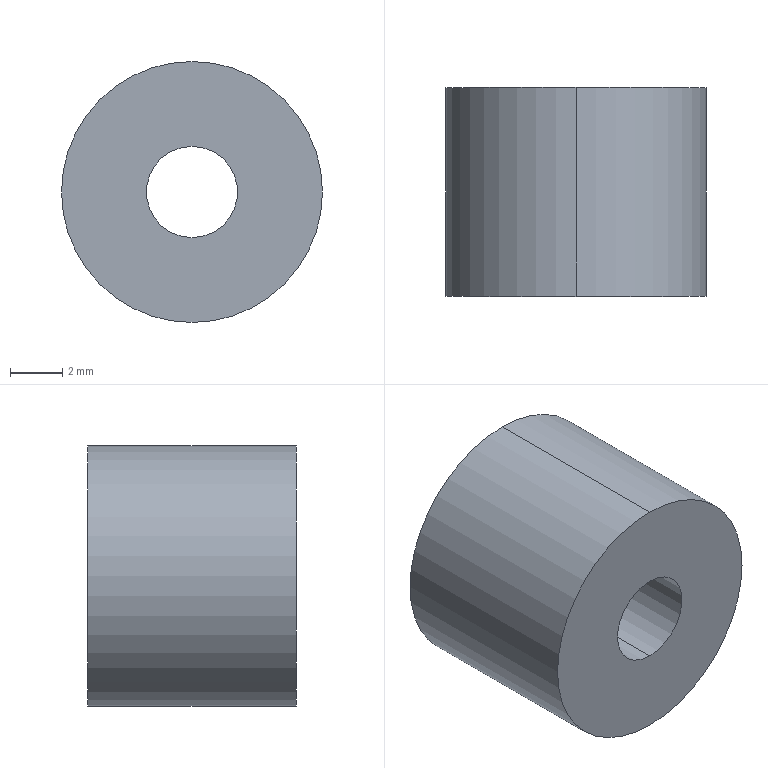Part | STEP file | PN_0011 | 1 solid | 9 faces | box 10 x 8 x 10 mm | volume 476.737 mm3 | cylinder 6 | plane 3 | commonest cylinder face diameters 3.5 x2 6 x2 10 x2
STEP:
#1=CARTESIAN_POINT('',(0.,0.,0.));
#2=DIRECTION('',(0.,0.,1.));
#3=DIRECTION('',(1.,0.,0.));
#4=AXIS2_PLACEMENT_3D('',#1,#2,#3);
#5=CARTESIAN_POINT('',(0.,8.,-3.));
#6=VERTEX_POINT('',#5);
#7=CARTESIAN_POINT('',(0.,4.,-3.));
#8=VERTEX_POINT('',#7);
#9=CARTESIAN_POINT('',(0.,0.,-3.));
#10=DIRECTION('',(0.,-1.,0.));
#11=VECTOR('',#10,1.);
#12=LINE('',#9,#11);
#13=CARTESIAN_POINT('',(0.,0.,0.));
#14=DIRECTION('',(0.,-1.,0.));
#15=DIRECTION('',(0.,0.,-1.));
#16=AXIS2_PLACEMENT_3D('',#13,#14,#15);
#17=CYLINDRICAL_SURFACE('',#16,3.);
#18=CARTESIAN_POINT('',(6.283,0.));
#19=DIRECTION('',(0.,1.));
#20=VECTOR('',#19,1.);
#21=LINE('',#18,#20);
#22=(GEOMETRIC_REPRESENTATION_CONTEXT(2)PARAMETRIC_REPRESENTATION_CONTEXT()REPRESENTATION_CONTEXT('',''));
#23=DEFINITIONAL_REPRESENTATION('',(#21),#22);
#24=PCURVE('',#17,#23);
#25=CARTESIAN_POINT('',(0.,0.,0.));
#26=DIRECTION('',(0.,-1.,0.));
#27=DIRECTION('',(0.,0.,-1.));
#28=AXIS2_PLACEMENT_3D('',#25,#26,#27);
#29=CYLINDRICAL_SURFACE('',#28,3.);
#30=CARTESIAN_POINT('',(0.,0.));
#31=DIRECTION('',(0.,1.));
#32=VECTOR('',#31,1.);
#33=LINE('',#30,#32);
#34=(GEOMETRIC_REPRESENTATION_CONTEXT(2)PARAMETRIC_REPRESENTATION_CONTEXT()REPRESENTATION_CONTEXT('',''));
#35=DEFINITIONAL_REPRESENTATION('',(#33),#34);
#36=PCURVE('',#29,#35);
#37=SURFACE_CURVE('',#12,(#24,#36),.PCURVE_S1.);
#38=EDGE_CURVE('',#6,#8,#37,.T.);
#39=ORIENTED_EDGE('',*,*,#38,.T.);
#40=CARTESIAN_POINT('',(0.,4.,3.));
#41=VERTEX_POINT('',#40);
#42=CARTESIAN_POINT('',(0.,4.,0.));
#43=DIRECTION('',(0.,-1.,0.));
#44=DIRECTION('',(0.,0.,-1.));
#45=AXIS2_PLACEMENT_3D('',#42,#43,#44);
#46=CIRCLE('',#45,3.);
#47=CARTESIAN_POINT('',(0.,-4.));
#48=DIRECTION('',(1.,0.));
#49=VECTOR('',#48,1.);
#50=LINE('',#47,#49);
#51=(GEOMETRIC_REPRESENTATION_CONTEXT(2)PARAMETRIC_REPRESENTATION_CONTEXT()REPRESENTATION_CONTEXT('',''));
#52=DEFINITIONAL_REPRESENTATION('',(#50),#51);
#53=PCURVE('',#17,#52);
#54=CARTESIAN_POINT('',(3.,4.,0.));
#55=DIRECTION('',(0.,1.,0.));
#56=DIRECTION('',(0.,0.,1.));
#57=AXIS2_PLACEMENT_3D('',#54,#55,#56);
#58=PLANE('',#57);
#59=CARTESIAN_POINT('',(-3.,-3.));
#60=CARTESIAN_POINT('',(-3.,2.196));
#61=CARTESIAN_POINT('',(1.5,-0.4019));
#62=CARTESIAN_POINT('',(6.,-3.));
#63=CARTESIAN_POINT('',(1.5,-5.598));
#64=CARTESIAN_POINT('',(-3.,-8.196));
#65=CARTESIAN_POINT('',(-3.,-3.));
#66=(BOUNDED_CURVE()B_SPLINE_CURVE(2,(#59,#60,#61,#62,#63,#64,#65),.UNSPECIFIED.,.T.,.F.)B_SPLINE_CURVE_WITH_KNOTS((1,2,2,2,2,1),(-2.094,0.,2.094,4.189,6.283,8.378),.UNSPECIFIED.)CURVE()GEOMETRIC_REPRESENTATION_ITEM()RATIONAL_B_SPLINE_CURVE((1.,0.5,1.,0.5,1.,0.5,1.))REPRESENTATION_ITEM(''));
#67=(GEOMETRIC_REPRESENTATION_CONTEXT(2)PARAMETRIC_REPRESENTATION_CONTEXT()REPRESENTATION_CONTEXT('',''));
#68=DEFINITIONAL_REPRESENTATION('',(#66),#67);
#69=PCURVE('',#58,#68);
#70=SURFACE_CURVE('',#46,(#53,#69),.PCURVE_S1.);
#71=EDGE_CURVE('',#41,#8,#70,.T.);
#72=ORIENTED_EDGE('',*,*,#71,.F.);
#73=CARTESIAN_POINT('',(0.,8.,3.));
#74=VERTEX_POINT('',#73);
#75=CARTESIAN_POINT('',(0.,0.,3.));
#76=DIRECTION('',(0.,-1.,0.));
#77=VECTOR('',#76,1.);
#78=LINE('',#75,#77);
#79=CARTESIAN_POINT('',(3.142,0.));
#80=DIRECTION('',(0.,1.));
#81=VECTOR('',#80,1.);
#82=LINE('',#79,#81);
#83=(GEOMETRIC_REPRESENTATION_CONTEXT(2)PARAMETRIC_REPRESENTATION_CONTEXT()REPRESENTATION_CONTEXT('',''));
#84=DEFINITIONAL_REPRESENTATION('',(#82),#83);
#85=PCURVE('',#17,#84);
#86=CARTESIAN_POINT('',(3.142,0.));
#87=DIRECTION('',(0.,1.));
#88=VECTOR('',#87,1.);
#89=LINE('',#86,#88);
#90=(GEOMETRIC_REPRESENTATION_CONTEXT(2)PARAMETRIC_REPRESENTATION_CONTEXT()REPRESENTATION_CONTEXT('',''));
#91=DEFINITIONAL_REPRESENTATION('',(#89),#90);
#92=PCURVE('',#29,#91);
#93=SURFACE_CURVE('',#78,(#85,#92),.PCURVE_S1.);
#94=EDGE_CURVE('',#74,#41,#93,.T.);
#95=ORIENTED_EDGE('',*,*,#94,.F.);
#96=CARTESIAN_POINT('',(0.,8.,0.));
#97=DIRECTION('',(0.,-1.,0.));
#98=DIRECTION('',(0.,0.,-1.));
#99=AXIS2_PLACEMENT_3D('',#96,#97,#98);
#100=CIRCLE('',#99,3.);
#101=CARTESIAN_POINT('',(0.,-8.));
#102=DIRECTION('',(1.,0.));
#103=VECTOR('',#102,1.);
#104=LINE('',#101,#103);
#105=(GEOMETRIC_REPRESENTATION_CONTEXT(2)PARAMETRIC_REPRESENTATION_CONTEXT()REPRESENTATION_CONTEXT('',''));
#106=DEFINITIONAL_REPRESENTATION('',(#104),#105);
#107=PCURVE('',#17,#106);
#108=CARTESIAN_POINT('',(3.,8.,0.));
#109=DIRECTION('',(0.,1.,0.));
#110=DIRECTION('',(0.,0.,1.));
#111=AXIS2_PLACEMENT_3D('',#108,#109,#110);
#112=PLANE('',#111);
#113=CARTESIAN_POINT('',(-3.,-3.));
#114=CARTESIAN_POINT('',(-3.,2.196));
#115=CARTESIAN_POINT('',(1.5,-0.4019));
#116=CARTESIAN_POINT('',(6.,-3.));
#117=CARTESIAN_POINT('',(1.5,-5.598));
#118=CARTESIAN_POINT('',(-3.,-8.196));
#119=CARTESIAN_POINT('',(-3.,-3.));
#120=(BOUNDED_CURVE()B_SPLINE_CURVE(2,(#113,#114,#115,#116,#117,#118,#119),.UNSPECIFIED.,.T.,.F.)B_SPLINE_CURVE_WITH_KNOTS((1,2,2,2,2,1),(-2.094,0.,2.094,4.189,6.283,8.378),.UNSPECIFIED.)CURVE()GEOMETRIC_REPRESENTATION_ITEM()RATIONAL_B_SPLINE_CURVE((1.,0.5,1.,0.5,1.,0.5,1.))REPRESENTATION_ITEM(''));
#121=(GEOMETRIC_REPRESENTATION_CONTEXT(2)PARAMETRIC_REPRESENTATION_CONTEXT()REPRESENTATION_CONTEXT('',''));
#122=DEFINITIONAL_REPRESENTATION('',(#120),#121);
#123=PCURVE('',#112,#122);
#124=SURFACE_CURVE('',#100,(#107,#123),.PCURVE_S1.);
#125=EDGE_CURVE('',#74,#6,#124,.T.);
#126=ORIENTED_EDGE('',*,*,#125,.T.);
#127=EDGE_LOOP('',(#39,#72,#95,#126));
#128=FACE_BOUND('',#127,.F.);
#129=ADVANCED_FACE('',(#128),#17,.F.);
#130=CARTESIAN_POINT('',(0.,4.,-1.75));
#131=VERTEX_POINT('',#130);
#132=CARTESIAN_POINT('',(0.,0.,-1.75));
#133=VERTEX_POINT('',#132);
#134=CARTESIAN_POINT('',(0.,0.,-1.75));
#135=DIRECTION('',(0.,-1.,0.));
#136=VECTOR('',#135,1.);
#137=LINE('',#134,#136);
#138=CARTESIAN_POINT('',(0.,0.,0.));
#139=DIRECTION('',(0.,-1.,0.));
#140=DIRECTION('',(0.,0.,-1.));
#141=AXIS2_PLACEMENT_3D('',#138,#139,#140);
#142=CYLINDRICAL_SURFACE('',#141,1.75);
#143=CARTESIAN_POINT('',(6.283,0.));
#144=DIRECTION('',(0.,1.));
#145=VECTOR('',#144,1.);
#146=LINE('',#143,#145);
#147=(GEOMETRIC_REPRESENTATION_CONTEXT(2)PARAMETRIC_REPRESENTATION_CONTEXT()REPRESENTATION_CONTEXT('',''));
#148=DEFINITIONAL_REPRESENTATION('',(#146),#147);
#149=PCURVE('',#142,#148);
#150=CARTESIAN_POINT('',(0.,0.,0.));
#151=DIRECTION('',(0.,-1.,0.));
#152=DIRECTION('',(0.,0.,-1.));
#153=AXIS2_PLACEMENT_3D('',#150,#151,#152);
#154=CYLINDRICAL_SURFACE('',#153,1.75);
#155=CARTESIAN_POINT('',(0.,0.));
#156=DIRECTION('',(0.,1.));
#157=VECTOR('',#156,1.);
#158=LINE('',#155,#157);
#159=(GEOMETRIC_REPRESENTATION_CONTEXT(2)PARAMETRIC_REPRESENTATION_CONTEXT()REPRESENTATION_CONTEXT('',''));
#160=DEFINITIONAL_REPRESENTATION('',(#158),#159);
#161=PCURVE('',#154,#160);
#162=SURFACE_CURVE('',#137,(#149,#161),.PCURVE_S1.);
#163=EDGE_CURVE('',#131,#133,#162,.T.);
#164=ORIENTED_EDGE('',*,*,#163,.T.);
#165=CARTESIAN_POINT('',(0.,0.,1.75));
#166=VERTEX_POINT('',#165);
#167=CARTESIAN_POINT('',(0.,0.,0.));
#168=DIRECTION('',(0.,-1.,0.));
#169=DIRECTION('',(0.,0.,-1.));
#170=AXIS2_PLACEMENT_3D('',#167,#168,#169);
#171=CIRCLE('',#170,1.75);
#172=CARTESIAN_POINT('',(0.,0.));
#173=DIRECTION('',(1.,0.));
#174=VECTOR('',#173,1.);
#175=LINE('',#172,#174);
#176=(GEOMETRIC_REPRESENTATION_CONTEXT(2)PARAMETRIC_REPRESENTATION_CONTEXT()REPRESENTATION_CONTEXT('',''));
#177=DEFINITIONAL_REPRESENTATION('',(#175),#176);
#178=PCURVE('',#142,#177);
#179=CARTESIAN_POINT('',(1.75,0.,0.));
#180=DIRECTION('',(0.,-1.,0.));
#181=DIRECTION('',(0.,0.,-1.));
#182=AXIS2_PLACEMENT_3D('',#179,#180,#181);
#183=PLANE('',#182);
#184=CARTESIAN_POINT('',(0.,-1.75));
#185=DIRECTION('',(1.,0.));
#186=AXIS2_PLACEMENT_2D('',#184,#185);
#187=CIRCLE('',#186,1.75);
#188=(GEOMETRIC_REPRESENTATION_CONTEXT(2)PARAMETRIC_REPRESENTATION_CONTEXT()REPRESENTATION_CONTEXT('',''));
#189=DEFINITIONAL_REPRESENTATION('',(#187),#188);
#190=PCURVE('',#183,#189);
#191=SURFACE_CURVE('',#171,(#178,#190),.PCURVE_S1.);
#192=EDGE_CURVE('',#166,#133,#191,.T.);
#193=ORIENTED_EDGE('',*,*,#192,.F.);
#194=CARTESIAN_POINT('',(0.,4.,1.75));
#195=VERTEX_POINT('',#194);
#196=CARTESIAN_POINT('',(0.,0.,1.75));
#197=DIRECTION('',(0.,-1.,0.));
#198=VECTOR('',#197,1.);
#199=LINE('',#196,#198);
#200=CARTESIAN_POINT('',(3.142,0.));
#201=DIRECTION('',(0.,1.));
#202=VECTOR('',#201,1.);
#203=LINE('',#200,#202);
#204=(GEOMETRIC_REPRESENTATION_CONTEXT(2)PARAMETRIC_REPRESENTATION_CONTEXT()REPRESENTATION_CONTEXT('',''));
#205=DEFINITIONAL_REPRESENTATION('',(#203),#204);
#206=PCURVE('',#142,#205);
#207=CARTESIAN_POINT('',(3.142,0.));
#208=DIRECTION('',(0.,1.));
#209=VECTOR('',#208,1.);
#210=LINE('',#207,#209);
#211=(GEOMETRIC_REPRESENTATION_CONTEXT(2)PARAMETRIC_REPRESENTATION_CONTEXT()REPRESENTATION_CONTEXT('',''));
#212=DEFINITIONAL_REPRESENTATION('',(#210),#211);
#213=PCURVE('',#154,#212);
#214=SURFACE_CURVE('',#199,(#206,#213),.PCURVE_S1.);
#215=EDGE_CURVE('',#195,#166,#214,.T.);
#216=ORIENTED_EDGE('',*,*,#215,.F.);
#217=CARTESIAN_POINT('',(0.,4.,0.));
#218=DIRECTION('',(0.,-1.,0.));
#219=DIRECTION('',(0.,0.,-1.));
#220=AXIS2_PLACEMENT_3D('',#217,#218,#219);
#221=CIRCLE('',#220,1.75);
#222=CARTESIAN_POINT('',(0.,-4.));
#223=DIRECTION('',(1.,0.));
#224=VECTOR('',#223,1.);
#225=LINE('',#222,#224);
#226=(GEOMETRIC_REPRESENTATION_CONTEXT(2)PARAMETRIC_REPRESENTATION_CONTEXT()REPRESENTATION_CONTEXT('',''));
#227=DEFINITIONAL_REPRESENTATION('',(#225),#226);
#228=PCURVE('',#142,#227);
#229=CARTESIAN_POINT('',(-1.75,-3.));
#230=CARTESIAN_POINT('',(-1.75,0.03109));
#231=CARTESIAN_POINT('',(0.875,-1.484));
#232=CARTESIAN_POINT('',(3.5,-3.));
#233=CARTESIAN_POINT('',(0.875,-4.516));
#234=CARTESIAN_POINT('',(-1.75,-6.031));
#235=CARTESIAN_POINT('',(-1.75,-3.));
#236=(BOUNDED_CURVE()B_SPLINE_CURVE(2,(#229,#230,#231,#232,#233,#234,#235),.UNSPECIFIED.,.T.,.F.)B_SPLINE_CURVE_WITH_KNOTS((1,2,2,2,2,1),(-2.094,0.,2.094,4.189,6.283,8.378),.UNSPECIFIED.)CURVE()GEOMETRIC_REPRESENTATION_ITEM()RATIONAL_B_SPLINE_CURVE((1.,0.5,1.,0.5,1.,0.5,1.))REPRESENTATION_ITEM(''));
#237=(GEOMETRIC_REPRESENTATION_CONTEXT(2)PARAMETRIC_REPRESENTATION_CONTEXT()REPRESENTATION_CONTEXT('',''));
#238=DEFINITIONAL_REPRESENTATION('',(#236),#237);
#239=PCURVE('',#58,#238);
#240=SURFACE_CURVE('',#221,(#228,#239),.PCURVE_S1.);
#241=EDGE_CURVE('',#195,#131,#240,.T.);
#242=ORIENTED_EDGE('',*,*,#241,.T.);
#243=EDGE_LOOP('',(#164,#193,#216,#242));
#244=FACE_BOUND('',#243,.F.);
#245=ADVANCED_FACE('',(#244),#142,.F.);
#246=CARTESIAN_POINT('',(0.,8.,-5.));
#247=VERTEX_POINT('',#246);
#248=CARTESIAN_POINT('',(0.,8.,5.));
#249=VERTEX_POINT('',#248);
#250=CARTESIAN_POINT('',(0.,8.,0.));
#251=DIRECTION('',(0.,-1.,0.));
#252=DIRECTION('',(0.,0.,-1.));
#253=AXIS2_PLACEMENT_3D('',#250,#251,#252);
#254=CIRCLE('',#253,5.);
#255=CARTESIAN_POINT('',(0.,0.,0.));
#256=DIRECTION('',(0.,-1.,0.));
#257=DIRECTION('',(0.,0.,-1.));
#258=AXIS2_PLACEMENT_3D('',#255,#256,#257);
#259=CYLINDRICAL_SURFACE('',#258,5.);
#260=CARTESIAN_POINT('',(0.,-8.));
#261=DIRECTION('',(1.,0.));
#262=VECTOR('',#261,1.);
#263=LINE('',#260,#262);
#264=(GEOMETRIC_REPRESENTATION_CONTEXT(2)PARAMETRIC_REPRESENTATION_CONTEXT()REPRESENTATION_CONTEXT('',''));
#265=DEFINITIONAL_REPRESENTATION('',(#263),#264);
#266=PCURVE('',#259,#265);
#267=CARTESIAN_POINT('',(-5.,-3.));
#268=CARTESIAN_POINT('',(-5.,5.66));
#269=CARTESIAN_POINT('',(2.5,1.33));
#270=CARTESIAN_POINT('',(10.,-3.));
#271=CARTESIAN_POINT('',(2.5,-7.33));
#272=CARTESIAN_POINT('',(-5.,-11.66));
#273=CARTESIAN_POINT('',(-5.,-3.));
#274=(BOUNDED_CURVE()B_SPLINE_CURVE(2,(#267,#268,#269,#270,#271,#272,#273),.UNSPECIFIED.,.T.,.F.)B_SPLINE_CURVE_WITH_KNOTS((1,2,2,2,2,1),(-2.094,0.,2.094,4.189,6.283,8.378),.UNSPECIFIED.)CURVE()GEOMETRIC_REPRESENTATION_ITEM()RATIONAL_B_SPLINE_CURVE((1.,0.5,1.,0.5,1.,0.5,1.))REPRESENTATION_ITEM(''));
#275=(GEOMETRIC_REPRESENTATION_CONTEXT(2)PARAMETRIC_REPRESENTATION_CONTEXT()REPRESENTATION_CONTEXT('',''));
#276=DEFINITIONAL_REPRESENTATION('',(#274),#275);
#277=PCURVE('',#112,#276);
#278=SURFACE_CURVE('',#254,(#266,#277),.PCURVE_S1.);
#279=EDGE_CURVE('',#247,#249,#278,.T.);
#280=ORIENTED_EDGE('',*,*,#279,.T.);
#281=CARTESIAN_POINT('',(0.,0.,5.));
#282=VERTEX_POINT('',#281);
#283=CARTESIAN_POINT('',(0.,0.,5.));
#284=DIRECTION('',(0.,-1.,0.));
#285=VECTOR('',#284,1.);
#286=LINE('',#283,#285);
#287=CARTESIAN_POINT('',(3.142,0.));
#288=DIRECTION('',(0.,1.));
#289=VECTOR('',#288,1.);
#290=LINE('',#287,#289);
#291=(GEOMETRIC_REPRESENTATION_CONTEXT(2)PARAMETRIC_REPRESENTATION_CONTEXT()REPRESENTATION_CONTEXT('',''));
#292=DEFINITIONAL_REPRESENTATION('',(#290),#291);
#293=PCURVE('',#259,#292);
#294=CARTESIAN_POINT('',(0.,0.,0.));
#295=DIRECTION('',(0.,-1.,0.));
#296=DIRECTION('',(0.,0.,-1.));
#297=AXIS2_PLACEMENT_3D('',#294,#295,#296);
#298=CYLINDRICAL_SURFACE('',#297,5.);
#299=CARTESIAN_POINT('',(3.142,0.));
#300=DIRECTION('',(0.,1.));
#301=VECTOR('',#300,1.);
#302=LINE('',#299,#301);
#303=(GEOMETRIC_REPRESENTATION_CONTEXT(2)PARAMETRIC_REPRESENTATION_CONTEXT()REPRESENTATION_CONTEXT('',''));
#304=DEFINITIONAL_REPRESENTATION('',(#302),#303);
#305=PCURVE('',#298,#304);
#306=SURFACE_CURVE('',#286,(#293,#305),.PCURVE_S1.);
#307=EDGE_CURVE('',#249,#282,#306,.T.);
#308=ORIENTED_EDGE('',*,*,#307,.T.);
#309=CARTESIAN_POINT('',(0.,0.,-5.));
#310=VERTEX_POINT('',#309);
#311=CARTESIAN_POINT('',(0.,0.,0.));
#312=DIRECTION('',(0.,-1.,0.));
#313=DIRECTION('',(0.,0.,-1.));
#314=AXIS2_PLACEMENT_3D('',#311,#312,#313);
#315=CIRCLE('',#314,5.);
#316=CARTESIAN_POINT('',(0.,0.));
#317=DIRECTION('',(1.,0.));
#318=VECTOR('',#317,1.);
#319=LINE('',#316,#318);
#320=(GEOMETRIC_REPRESENTATION_CONTEXT(2)PARAMETRIC_REPRESENTATION_CONTEXT()REPRESENTATION_CONTEXT('',''));
#321=DEFINITIONAL_REPRESENTATION('',(#319),#320);
#322=PCURVE('',#259,#321);
#323=CARTESIAN_POINT('',(0.,-1.75));
#324=DIRECTION('',(1.,0.));
#325=AXIS2_PLACEMENT_2D('',#323,#324);
#326=CIRCLE('',#325,5.);
#327=(GEOMETRIC_REPRESENTATION_CONTEXT(2)PARAMETRIC_REPRESENTATION_CONTEXT()REPRESENTATION_CONTEXT('',''));
#328=DEFINITIONAL_REPRESENTATION('',(#326),#327);
#329=PCURVE('',#183,#328);
#330=SURFACE_CURVE('',#315,(#322,#329),.PCURVE_S1.);
#331=EDGE_CURVE('',#310,#282,#330,.T.);
#332=ORIENTED_EDGE('',*,*,#331,.F.);
#333=CARTESIAN_POINT('',(0.,0.,-5.));
#334=DIRECTION('',(0.,-1.,0.));
#335=VECTOR('',#334,1.);
#336=LINE('',#333,#335);
#337=CARTESIAN_POINT('',(0.,0.));
#338=DIRECTION('',(0.,1.));
#339=VECTOR('',#338,1.);
#340=LINE('',#337,#339);
#341=(GEOMETRIC_REPRESENTATION_CONTEXT(2)PARAMETRIC_REPRESENTATION_CONTEXT()REPRESENTATION_CONTEXT('',''));
#342=DEFINITIONAL_REPRESENTATION('',(#340),#341);
#343=PCURVE('',#259,#342);
#344=CARTESIAN_POINT('',(6.283,0.));
#345=DIRECTION('',(0.,1.));
#346=VECTOR('',#345,1.);
#347=LINE('',#344,#346);
#348=(GEOMETRIC_REPRESENTATION_CONTEXT(2)PARAMETRIC_REPRESENTATION_CONTEXT()REPRESENTATION_CONTEXT('',''));
#349=DEFINITIONAL_REPRESENTATION('',(#347),#348);
#350=PCURVE('',#298,#349);
#351=SURFACE_CURVE('',#336,(#343,#350),.PCURVE_S1.);
#352=EDGE_CURVE('',#247,#310,#351,.T.);
#353=ORIENTED_EDGE('',*,*,#352,.F.);
#354=EDGE_LOOP('',(#280,#308,#332,#353));
#355=FACE_BOUND('',#354,.T.);
#356=ADVANCED_FACE('',(#355),#259,.T.);
#357=ORIENTED_EDGE('',*,*,#307,.F.);
#358=CARTESIAN_POINT('',(0.,8.,0.));
#359=DIRECTION('',(0.,-1.,0.));
#360=DIRECTION('',(0.,0.,-1.));
#361=AXIS2_PLACEMENT_3D('',#358,#359,#360);
#362=CIRCLE('',#361,5.);
#363=CARTESIAN_POINT('',(0.,-8.));
#364=DIRECTION('',(1.,0.));
#365=VECTOR('',#364,1.);
#366=LINE('',#363,#365);
#367=(GEOMETRIC_REPRESENTATION_CONTEXT(2)PARAMETRIC_REPRESENTATION_CONTEXT()REPRESENTATION_CONTEXT('',''));
#368=DEFINITIONAL_REPRESENTATION('',(#366),#367);
#369=PCURVE('',#298,#368);
#370=CARTESIAN_POINT('',(-5.,-3.));
#371=CARTESIAN_POINT('',(-5.,5.66));
#372=CARTESIAN_POINT('',(2.5,1.33));
#373=CARTESIAN_POINT('',(10.,-3.));
#374=CARTESIAN_POINT('',(2.5,-7.33));
#375=CARTESIAN_POINT('',(-5.,-11.66));
#376=CARTESIAN_POINT('',(-5.,-3.));
#377=(BOUNDED_CURVE()B_SPLINE_CURVE(2,(#370,#371,#372,#373,#374,#375,#376),.UNSPECIFIED.,.T.,.F.)B_SPLINE_CURVE_WITH_KNOTS((1,2,2,2,2,1),(-2.094,0.,2.094,4.189,6.283,8.378),.UNSPECIFIED.)CURVE()GEOMETRIC_REPRESENTATION_ITEM()RATIONAL_B_SPLINE_CURVE((1.,0.5,1.,0.5,1.,0.5,1.))REPRESENTATION_ITEM(''));
#378=(GEOMETRIC_REPRESENTATION_CONTEXT(2)PARAMETRIC_REPRESENTATION_CONTEXT()REPRESENTATION_CONTEXT('',''));
#379=DEFINITIONAL_REPRESENTATION('',(#377),#378);
#380=PCURVE('',#112,#379);
#381=SURFACE_CURVE('',#362,(#369,#380),.PCURVE_S1.);
#382=EDGE_CURVE('',#249,#247,#381,.T.);
#383=ORIENTED_EDGE('',*,*,#382,.T.);
#384=ORIENTED_EDGE('',*,*,#352,.T.);
#385=CARTESIAN_POINT('',(0.,0.,0.));
#386=DIRECTION('',(0.,-1.,0.));
#387=DIRECTION('',(0.,0.,-1.));
#388=AXIS2_PLACEMENT_3D('',#385,#386,#387);
#389=CIRCLE('',#388,5.);
#390=CARTESIAN_POINT('',(0.,0.));
#391=DIRECTION('',(1.,0.));
#392=VECTOR('',#391,1.);
#393=LINE('',#390,#392);
#394=(GEOMETRIC_REPRESENTATION_CONTEXT(2)PARAMETRIC_REPRESENTATION_CONTEXT()REPRESENTATION_CONTEXT('',''));
#395=DEFINITIONAL_REPRESENTATION('',(#393),#394);
#396=PCURVE('',#298,#395);
#397=CARTESIAN_POINT('',(0.,-1.75));
#398=DIRECTION('',(1.,0.));
#399=AXIS2_PLACEMENT_2D('',#397,#398);
#400=CIRCLE('',#399,5.);
#401=(GEOMETRIC_REPRESENTATION_CONTEXT(2)PARAMETRIC_REPRESENTATION_CONTEXT()REPRESENTATION_CONTEXT('',''));
#402=DEFINITIONAL_REPRESENTATION('',(#400),#401);
#403=PCURVE('',#183,#402);
#404=SURFACE_CURVE('',#389,(#396,#403),.PCURVE_S1.);
#405=EDGE_CURVE('',#282,#310,#404,.T.);
#406=ORIENTED_EDGE('',*,*,#405,.F.);
#407=EDGE_LOOP('',(#357,#383,#384,#406));
#408=FACE_BOUND('',#407,.T.);
#409=ADVANCED_FACE('',(#408),#298,.T.);
#410=ORIENTED_EDGE('',*,*,#331,.T.);
#411=ORIENTED_EDGE('',*,*,#405,.T.);
#412=EDGE_LOOP('',(#410,#411));
#413=FACE_BOUND('',#412,.T.);
#414=CARTESIAN_POINT('',(0.,0.,0.));
#415=DIRECTION('',(0.,-1.,0.));
#416=DIRECTION('',(0.,0.,-1.));
#417=AXIS2_PLACEMENT_3D('',#414,#415,#416);
#418=CIRCLE('',#417,1.75);
#419=CARTESIAN_POINT('',(0.,-1.75));
#420=DIRECTION('',(1.,0.));
#421=AXIS2_PLACEMENT_2D('',#419,#420);
#422=CIRCLE('',#421,1.75);
#423=(GEOMETRIC_REPRESENTATION_CONTEXT(2)PARAMETRIC_REPRESENTATION_CONTEXT()REPRESENTATION_CONTEXT('',''));
#424=DEFINITIONAL_REPRESENTATION('',(#422),#423);
#425=PCURVE('',#183,#424);
#426=CARTESIAN_POINT('',(0.,0.));
#427=DIRECTION('',(1.,0.));
#428=VECTOR('',#427,1.);
#429=LINE('',#426,#428);
#430=(GEOMETRIC_REPRESENTATION_CONTEXT(2)PARAMETRIC_REPRESENTATION_CONTEXT()REPRESENTATION_CONTEXT('',''));
#431=DEFINITIONAL_REPRESENTATION('',(#429),#430);
#432=PCURVE('',#154,#431);
#433=SURFACE_CURVE('',#418,(#425,#432),.PCURVE_S1.);
#434=EDGE_CURVE('',#133,#166,#433,.T.);
#435=ORIENTED_EDGE('',*,*,#434,.F.);
#436=ORIENTED_EDGE('',*,*,#192,.F.);
#437=EDGE_LOOP('',(#435,#436));
#438=FACE_BOUND('',#437,.T.);
#439=ADVANCED_FACE('',(#413,#438),#183,.T.);
#440=ORIENTED_EDGE('',*,*,#434,.F.);
#441=ORIENTED_EDGE('',*,*,#163,.F.);
#442=CARTESIAN_POINT('',(0.,4.,0.));
#443=DIRECTION('',(0.,-1.,0.));
#444=DIRECTION('',(0.,0.,-1.));
#445=AXIS2_PLACEMENT_3D('',#442,#443,#444);
#446=CIRCLE('',#445,1.75);
#447=CARTESIAN_POINT('',(0.,-4.));
#448=DIRECTION('',(1.,0.));
#449=VECTOR('',#448,1.);
#450=LINE('',#447,#449);
#451=(GEOMETRIC_REPRESENTATION_CONTEXT(2)PARAMETRIC_REPRESENTATION_CONTEXT()REPRESENTATION_CONTEXT('',''));
#452=DEFINITIONAL_REPRESENTATION('',(#450),#451);
#453=PCURVE('',#154,#452);
#454=CARTESIAN_POINT('',(-1.75,-3.));
#455=CARTESIAN_POINT('',(-1.75,0.03109));
#456=CARTESIAN_POINT('',(0.875,-1.484));
#457=CARTESIAN_POINT('',(3.5,-3.));
#458=CARTESIAN_POINT('',(0.875,-4.516));
#459=CARTESIAN_POINT('',(-1.75,-6.031));
#460=CARTESIAN_POINT('',(-1.75,-3.));
#461=(BOUNDED_CURVE()B_SPLINE_CURVE(2,(#454,#455,#456,#457,#458,#459,#460),.UNSPECIFIED.,.T.,.F.)B_SPLINE_CURVE_WITH_KNOTS((1,2,2,2,2,1),(-2.094,0.,2.094,4.189,6.283,8.378),.UNSPECIFIED.)CURVE()GEOMETRIC_REPRESENTATION_ITEM()RATIONAL_B_SPLINE_CURVE((1.,0.5,1.,0.5,1.,0.5,1.))REPRESENTATION_ITEM(''));
#462=(GEOMETRIC_REPRESENTATION_CONTEXT(2)PARAMETRIC_REPRESENTATION_CONTEXT()REPRESENTATION_CONTEXT('',''));
#463=DEFINITIONAL_REPRESENTATION('',(#461),#462);
#464=PCURVE('',#58,#463);
#465=SURFACE_CURVE('',#446,(#453,#464),.PCURVE_S1.);
#466=EDGE_CURVE('',#131,#195,#465,.T.);
#467=ORIENTED_EDGE('',*,*,#466,.T.);
#468=ORIENTED_EDGE('',*,*,#215,.T.);
#469=EDGE_LOOP('',(#440,#441,#467,#468));
#470=FACE_BOUND('',#469,.F.);
#471=ADVANCED_FACE('',(#470),#154,.F.);
#472=ORIENTED_EDGE('',*,*,#466,.T.);
#473=ORIENTED_EDGE('',*,*,#241,.T.);
#474=EDGE_LOOP('',(#472,#473));
#475=FACE_BOUND('',#474,.T.);
#476=CARTESIAN_POINT('',(0.,4.,0.));
#477=DIRECTION('',(0.,-1.,0.));
#478=DIRECTION('',(0.,0.,-1.));
#479=AXIS2_PLACEMENT_3D('',#476,#477,#478);
#480=CIRCLE('',#479,3.);
#481=CARTESIAN_POINT('',(-3.,-3.));
#482=CARTESIAN_POINT('',(-3.,2.196));
#483=CARTESIAN_POINT('',(1.5,-0.4019));
#484=CARTESIAN_POINT('',(6.,-3.));
#485=CARTESIAN_POINT('',(1.5,-5.598));
#486=CARTESIAN_POINT('',(-3.,-8.196));
#487=CARTESIAN_POINT('',(-3.,-3.));
#488=(BOUNDED_CURVE()B_SPLINE_CURVE(2,(#481,#482,#483,#484,#485,#486,#487),.UNSPECIFIED.,.T.,.F.)B_SPLINE_CURVE_WITH_KNOTS((1,2,2,2,2,1),(-2.094,0.,2.094,4.189,6.283,8.378),.UNSPECIFIED.)CURVE()GEOMETRIC_REPRESENTATION_ITEM()RATIONAL_B_SPLINE_CURVE((1.,0.5,1.,0.5,1.,0.5,1.))REPRESENTATION_ITEM(''));
#489=(GEOMETRIC_REPRESENTATION_CONTEXT(2)PARAMETRIC_REPRESENTATION_CONTEXT()REPRESENTATION_CONTEXT('',''));
#490=DEFINITIONAL_REPRESENTATION('',(#488),#489);
#491=PCURVE('',#58,#490);
#492=CARTESIAN_POINT('',(0.,-4.));
#493=DIRECTION('',(1.,0.));
#494=VECTOR('',#493,1.);
#495=LINE('',#492,#494);
#496=(GEOMETRIC_REPRESENTATION_CONTEXT(2)PARAMETRIC_REPRESENTATION_CONTEXT()REPRESENTATION_CONTEXT('',''));
#497=DEFINITIONAL_REPRESENTATION('',(#495),#496);
#498=PCURVE('',#29,#497);
#499=SURFACE_CURVE('',#480,(#491,#498),.PCURVE_S1.);
#500=EDGE_CURVE('',#8,#41,#499,.T.);
#501=ORIENTED_EDGE('',*,*,#500,.F.);
#502=ORIENTED_EDGE('',*,*,#71,.F.);
#503=EDGE_LOOP('',(#501,#502));
#504=FACE_BOUND('',#503,.T.);
#505=ADVANCED_FACE('',(#475,#504),#58,.T.);
#506=ORIENTED_EDGE('',*,*,#500,.F.);
#507=ORIENTED_EDGE('',*,*,#38,.F.);
#508=CARTESIAN_POINT('',(0.,8.,0.));
#509=DIRECTION('',(0.,-1.,0.));
#510=DIRECTION('',(0.,0.,-1.));
#511=AXIS2_PLACEMENT_3D('',#508,#509,#510);
#512=CIRCLE('',#511,3.);
#513=CARTESIAN_POINT('',(0.,-8.));
#514=DIRECTION('',(1.,0.));
#515=VECTOR('',#514,1.);
#516=LINE('',#513,#515);
#517=(GEOMETRIC_REPRESENTATION_CONTEXT(2)PARAMETRIC_REPRESENTATION_CONTEXT()REPRESENTATION_CONTEXT('',''));
#518=DEFINITIONAL_REPRESENTATION('',(#516),#517);
#519=PCURVE('',#29,#518);
#520=CARTESIAN_POINT('',(-3.,-3.));
#521=CARTESIAN_POINT('',(-3.,2.196));
#522=CARTESIAN_POINT('',(1.5,-0.4019));
#523=CARTESIAN_POINT('',(6.,-3.));
#524=CARTESIAN_POINT('',(1.5,-5.598));
#525=CARTESIAN_POINT('',(-3.,-8.196));
#526=CARTESIAN_POINT('',(-3.,-3.));
#527=(BOUNDED_CURVE()B_SPLINE_CURVE(2,(#520,#521,#522,#523,#524,#525,#526),.UNSPECIFIED.,.T.,.F.)B_SPLINE_CURVE_WITH_KNOTS((1,2,2,2,2,1),(-2.094,0.,2.094,4.189,6.283,8.378),.UNSPECIFIED.)CURVE()GEOMETRIC_REPRESENTATION_ITEM()RATIONAL_B_SPLINE_CURVE((1.,0.5,1.,0.5,1.,0.5,1.))REPRESENTATION_ITEM(''));
#528=(GEOMETRIC_REPRESENTATION_CONTEXT(2)PARAMETRIC_REPRESENTATION_CONTEXT()REPRESENTATION_CONTEXT('',''));
#529=DEFINITIONAL_REPRESENTATION('',(#527),#528);
#530=PCURVE('',#112,#529);
#531=SURFACE_CURVE('',#512,(#519,#530),.PCURVE_S1.);
#532=EDGE_CURVE('',#6,#74,#531,.T.);
#533=ORIENTED_EDGE('',*,*,#532,.T.);
#534=ORIENTED_EDGE('',*,*,#94,.T.);
#535=EDGE_LOOP('',(#506,#507,#533,#534));
#536=FACE_BOUND('',#535,.F.);
#537=ADVANCED_FACE('',(#536),#29,.F.);
#538=ORIENTED_EDGE('',*,*,#532,.T.);
#539=ORIENTED_EDGE('',*,*,#125,.T.);
#540=EDGE_LOOP('',(#538,#539));
#541=FACE_BOUND('',#540,.T.);
#542=ORIENTED_EDGE('',*,*,#279,.F.);
#543=ORIENTED_EDGE('',*,*,#382,.F.);
#544=EDGE_LOOP('',(#542,#543));
#545=FACE_BOUND('',#544,.T.);
#546=ADVANCED_FACE('',(#541,#545),#112,.T.);
#547=CLOSED_SHELL('',(#129,#245,#356,#409,#439,#471,#505,#537,#546));
#548=MANIFOLD_SOLID_BREP('',#547);
#549=(LENGTH_UNIT()NAMED_UNIT(*)SI_UNIT(.MILLI.,.METRE.));
#550=UNCERTAINTY_MEASURE_WITH_UNIT(LENGTH_MEASURE(0.0000001),#549,'','');
#551=(NAMED_UNIT(*)PLANE_ANGLE_UNIT()SI_UNIT($,.RADIAN.));
#552=(NAMED_UNIT(*)SI_UNIT($,.STERADIAN.)SOLID_ANGLE_UNIT());
#553=(GEOMETRIC_REPRESENTATION_CONTEXT(3)GLOBAL_UNCERTAINTY_ASSIGNED_CONTEXT((#550))GLOBAL_UNIT_ASSIGNED_CONTEXT((#549,#551,#552))REPRESENTATION_CONTEXT('',''));
#554=ADVANCED_BREP_SHAPE_REPRESENTATION('',(#4,#548),#553);